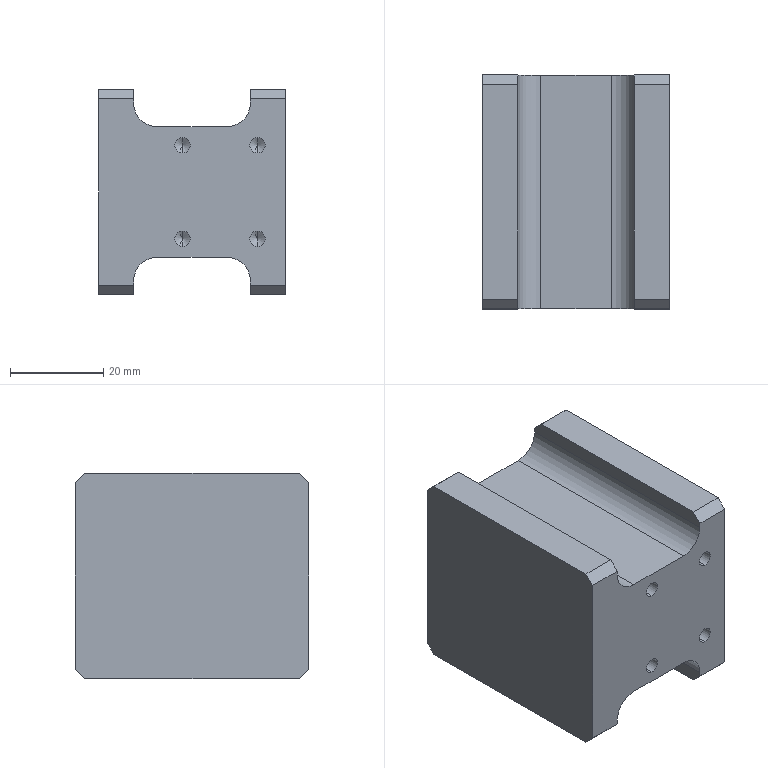Part | SolidWorks | features HoleWzd 3, ICE 2, Chamfer 1, CirPattern 1, Extrusion 1, Fillet 1 | 1 solid | 65 faces | box 40 x 50 x 44 mm | volume 66825 mm3 | cylinder 24 | plane 23 | cone 18 | commonest cylinder face diameters 2.5 x10 3.3 x8 10 x6